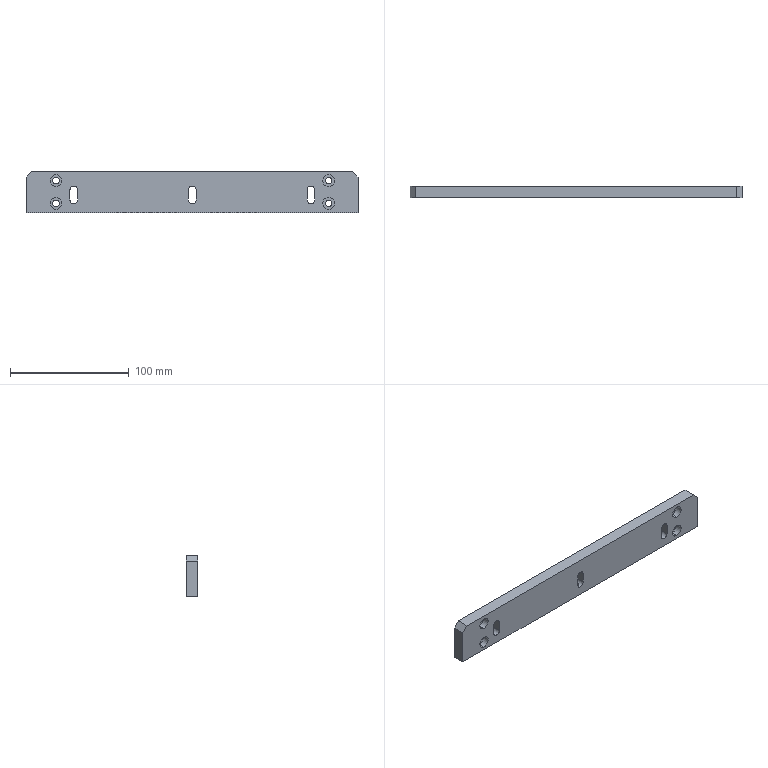Part | STEP file | PN_0034 | 1 solid | 61 faces | box 280 x 10 x 35 mm | volume 92081 mm3 | cylinder 35 | plane 18 | cone 8 | commonest cylinder face diameters 4.2 x10 6.5 x9 5.5 x8 10 x8